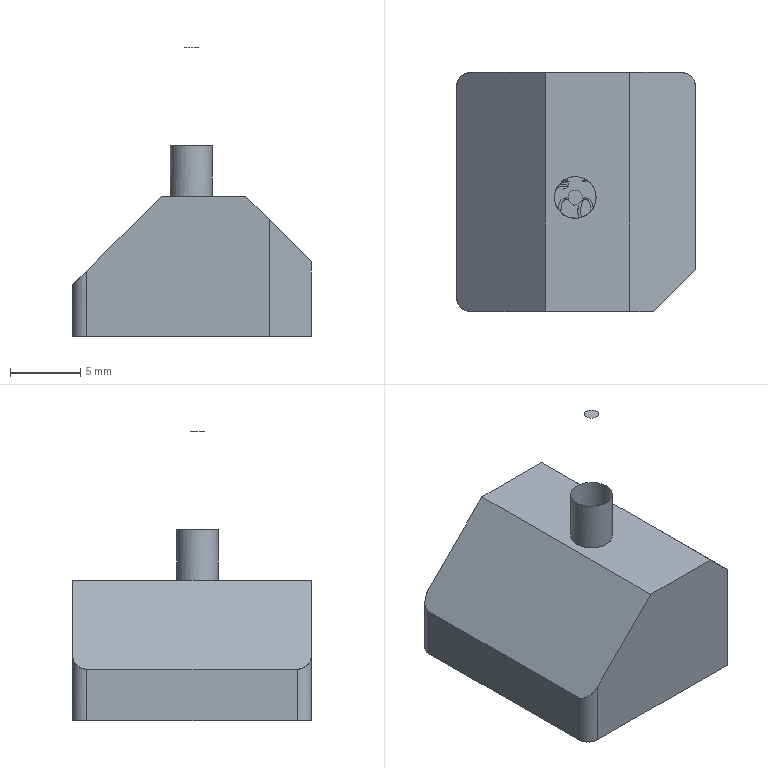NC program | PowerMill | posted with a generic post | part box 17 x 17 x 20.603 mm
Lines 1 to 1061 of 69435:
%
O0001
N104 ( POWERMILL CB  : 2026004.0)
N105 ( POST VER      : 2026.0.0.5161)
N106 ( OPTION FILE   : FANUC)
N107 ( OUTPUT WORKPLANE : WORLD)
N108 (  )
N109 ( TOOL LIST )
N110 (---------------------------------------)
N111 ( NO. | ID        | DIA.| TIP RAD|LENGTH)
N112 (---------------------------------------)
N113 (    1|D10C_1_1_1 |10.0 |  0.0   |76.04 )
N114 (    3|D10_1_1_1  |10.0 |  0.0   |75.76 )
N115 (   14|D4_1_1     | 4.0 |  0.0   |65.76 )
N116 (    7|R2_1_1     | 4.0 |  2.0   | 73.2 )
N117 (   13|TEXT_D4_1_1| 4.0 |  0.3   |65.88 )
N118 (---------------------------------------)
N119 (  )
N120 ( NUMBER OF TOOLPATHS: 10.0 )
N121 ( ESTIMATED PROGRAM DURATION: 0 HOURS 6 MIN 42 SEC)
N122 (  )
N123 G00 G21 G80 G40 G17
N124 G90
N125 G54
N126 G53 Z0.0
N127 (---------------)
N128 ( START TOOLPATH : 精公开粗01-扫面平行-D10C )
N129 (---------------)
N130 ( TOOL NO.    :1 )
N131 ( TOOL TYPE   : ENDMILL)
N132 ( TOOL ID     : D10C_1_1_1)
N133 ( TOOL DIA    : 10.0 LENGTH 76.04)
N134 T1
N135 M6
N136 S8000 M03
N137 G00 G90 X0.002 Y0.0
N138 G43 Z10.2 H1
N139
N140 G05 P10000 R4
N141 X16.302 Y11.3
N142 Z1.153
N143 G01 Z-0.047 F6000.0
N144 X11.302 F10000.0
N145 X-11.298
N146 Y5.65
N147 X11.302
N148 Y0.0
N149 X-11.298
N150 Y-5.65
N151 X11.302
N152 Y-11.3
N153 X-11.298
N154 X-16.298
N155 G00 Z10.2
N156 G05 P0
N157 (---------------)
N158 ( END TOOLPATH : 精公开粗01-扫面平行-D10C )
N159 (---------------)
N160 ( START TOOLPATH : 精公开粗01-外形偏置-D10C )
N161 (---------------)
N162 G00 X0.002 Y0.0 Z9.903
N163 G05 P10000 R4
N164 X5.2155 Y-16.575
N165 Z0.7136
N166 G01 Z-0.4864 F6000.0
N167 Y-16.0475 F10000.0
N168 G03 X0.468 Y-11.3 I-4.7475 J0.0
N169 G01 X-10.298
N170 G02 X-11.298 Y-10.3 I0.0 J1.0
N171 G01 Y10.3
N172 G02 X-10.298 Y11.3 I1.0 J0.0
N173 G01 X10.302
N174 G02 X11.302 Y10.3 I0.0 J-1.0
N175 G01 Y-10.3
N176 G02 X10.302 Y-11.3 I-1.0 J0.0
N177 G01 X0.468
N178 X0.3887 Y-6.22
N179 X-0.3847 Y-6.2321
N180 X-1.1581 Y-6.1315
N181 X-1.9316 Y-5.9309
N182 X-2.2756 Y-5.8007
N183 X-2.705 Y-5.5991
N184 X-3.4784 Y-5.1313
N185 X-4.2518 Y-4.4575
N186 X-4.4418 Y-4.2538
N187 X-5.0102 Y-3.4804
N188 X-5.4189 Y-2.707
N189 X-5.684 Y-1.9336
N190 X-5.8444 Y-1.1601
N191 X-5.889 Y-0.3867
N192 X-5.8408 Y0.3867
N193 X-5.6766 Y1.1601
N194 X-5.4075 Y1.9336
N195 X-5.0253 Y2.6552
N196 X-4.4176 Y3.4804
N197 X-4.2518 Y3.6568
N198 X-3.5825 Y4.2538
N199 X-2.705 Y4.7989
N200 X-1.9316 Y5.1308
N201 X-1.1581 Y5.3315
N202 X-0.3847 Y5.4321
N203 X0.3887 Y5.42
N204 X1.1621 Y5.3138
N205 X1.9356 Y5.0877
N206 X2.709 Y4.7473
N207 X3.4724 Y4.2538
N208 X4.2558 Y3.5415
N209 X4.894 Y2.707
N210 X5.2973 Y1.9336
N211 X5.5769 Y1.1601
N212 X5.7309 Y0.3867
N213 X5.7892 Y-0.3867
N214 X5.7346 Y-1.1601
N215 X5.5841 Y-1.9336
N216 X5.3099 Y-2.707
N217 X4.9107 Y-3.4804
N218 X4.3331 Y-4.2538
N219 X3.508 Y-5.0273
N220 X2.709 Y-5.5476
N221 X2.1672 Y-5.8007
N222 X1.1621 Y-6.1139
N223 X0.3887 Y-6.22
N224 X0.468 Y-11.3
N225 G00 Z3.3243
N226 G01 X5.2155 Y-16.575
N227 G00 Z0.3243
N228 G01 Z-0.8757 F6000.0
N229 Y-16.0475 F10000.0
N230 G03 X0.468 Y-11.3 I-4.7475 J0.0
N231 G01 X-10.298
N232 G02 X-11.298 Y-10.3 I0.0 J1.0
N233 G01 Y10.3
N234 G02 X-10.298 Y11.3 I1.0 J0.0
N235 G01 X10.302
N236 G02 X11.302 Y10.3 I0.0 J-1.0
N237 G01 Y-10.3
N238 G02 X10.302 Y-11.3 I-1.0 J0.0
N239 G01 X0.47
N240 X0.3887 Y-6.2744
N241 X-0.3847 Y-6.2869
N242 X-1.1581 Y-6.1868
N243 X-1.9316 Y-5.9885
N244 X-2.4138 Y-5.8007
N245 X-2.705 Y-5.6602
N246 X-3.4784 Y-5.1988
N247 X-3.7048 Y-5.0273
N248 X-4.2518 Y-4.5338
N249 X-4.514 Y-4.2538
N250 X-5.0253 Y-3.5593
N251 X-5.478 Y-2.707
N252 X-5.7402 Y-1.9336
N253 X-5.8995 Y-1.1601
N254 X-5.9432 Y-0.3867
N255 X-5.896 Y0.3867
N256 X-5.7987 Y0.9095
N257 X-5.4671 Y1.9336
N258 X-5.0573 Y2.707
N259 X-4.4901 Y3.4804
N260 X-4.2518 Y3.7337
N261 X-3.6709 Y4.2538
N262 X-3.4784 Y4.3979
N263 X-2.705 Y4.8597
N264 X-2.3533 Y5.0273
N265 X-1.9316 Y5.1882
N266 X-1.1581 Y5.3868
N267 X-0.3847 Y5.4869
N268 X0.3887 Y5.4744
N269 X1.1621 Y5.3695
N270 X1.9356 Y5.1452
N271 X2.2472 Y5.0273
N272 X2.709 Y4.809
N273 X3.4824 Y4.3143
N274 X4.2558 Y3.6223
N275 X4.9581 Y2.707
N276 X5.3562 Y1.9336
N277 X5.6333 Y1.1601
N278 X5.7856 Y0.3867
N279 X5.8439 Y-0.3867
N280 X5.8027 Y-1.0591
N281 X5.6405 Y-1.9336
N282 X5.3687 Y-2.707
N283 X5.0293 Y-3.3898
N284 X4.4041 Y-4.2538
N285 X4.2558 Y-4.4219
N286 X3.5976 Y-5.0273
N287 X2.709 Y-5.6096
N288 X2.3098 Y-5.8007
N289 X1.9356 Y-5.9451
N290 X1.1621 Y-6.1696
N291 X0.3887 Y-6.2744
N292 X0.47 Y-11.3
N293 X0.468
N294 G00 Z2.9349
N295 G01 X5.2155 Y-16.575
N296 G00 Z-0.0651
N297 G01 Z-1.2651 F6000.0
N298 Y-16.0475 F10000.0
N299 G03 X0.468 Y-11.3 I-4.7475 J0.0
N300 G01 X-10.298
N301 G02 X-11.298 Y-10.3 I0.0 J1.0
N302 G01 Y10.3
N303 G02 X-10.298 Y11.3 I1.0 J0.0
N304 G01 X10.302
N305 G02 X11.302 Y10.3 I0.0 J-1.0
N306 G01 Y-10.3
N307 G02 X10.302 Y-11.3 I-1.0 J0.0
N308 G01 X0.472
N309 X0.3887 Y-6.3287
N310 X-0.3847 Y-6.3417
N311 X-1.1581 Y-6.2421
N312 X-1.9316 Y-6.0461
N313 X-2.5431 Y-5.8007
N314 X-3.4784 Y-5.2654
N315 X-3.7912 Y-5.0273
N316 X-4.2518 Y-4.6101
N317 X-4.5858 Y-4.2538
N318 X-5.0253 Y-3.6611
N319 X-5.5372 Y-2.707
N320 X-5.7965 Y-1.9336
N321 X-5.9547 Y-1.1601
N322 X-5.9974 Y-0.3867
N323 X-5.9512 Y0.3867
N324 X-5.7987 Y1.1257
N325 X-5.5266 Y1.9336
N326 X-5.1207 Y2.707
N327 X-4.5626 Y3.4804
N328 X-4.2518 Y3.8107
N329 X-3.7589 Y4.2538
N330 X-3.4784 Y4.4648
N331 X-2.705 Y4.9204
N332 X-1.9316 Y5.2456
N333 X-1.1581 Y5.4421
N334 X-0.3847 Y5.5417
N335 X0.3887 Y5.5287
N336 X1.1621 Y5.4252
N337 X1.9356 Y5.2027
N338 X2.3859 Y5.0273
N339 X2.709 Y4.8706
N340 X3.653 Y4.2538
N341 X4.2558 Y3.703
N342 X4.4529 Y3.4804
N343 X5.0221 Y2.707
N344 X5.4151 Y1.9336
N345 X5.6898 Y1.1601
N346 X5.8027 Y0.6452
N347 X5.8986 Y-0.3867
N348 X5.844 Y-1.1601
N349 X5.6969 Y-1.9336
N350 X5.4274 Y-2.707
N351 X5.0383 Y-3.4804
N352 X4.4751 Y-4.2538
N353 X4.2558 Y-4.5022
N354 X3.6863 Y-5.0273
N355 X3.4824 Y-5.1815
N356 X2.709 Y-5.6716
N357 X2.4438 Y-5.8007
N358 X1.9356 Y-6.0026
N359 X1.1621 Y-6.2253
N360 X0.3887 Y-6.3287
N361 X0.472 Y-11.3
N362 X0.468
N363 G00 Z2.5455
N364 G01 X5.2155 Y-16.575
N365 G00 Z-0.4545
N366 G01 Z-1.6545 F6000.0
N367 Y-16.0475 F10000.0
N368 G03 X0.468 Y-11.3 I-4.7475 J0.0
N369 G01 X-10.298
N370 G02 X-11.298 Y-10.3 I0.0 J1.0
N371 G01 Y10.3
N372 G02 X-10.298 Y11.3 I1.0 J0.0
N373 G01 X10.302
N374 G02 X11.302 Y10.3 I0.0 J-1.0
N375 G01 Y-10.3
N376 G02 X10.302 Y-11.3 I-1.0 J0.0
N377 G01 X0.4739
N378 X0.3887 Y-6.3831
N379 X-0.3847 Y-6.3965
N380 X-1.1581 Y-6.2975
N381 X-1.9316 Y-6.1036
N382 X-2.6679 Y-5.8007
N383 X-3.4784 Y-5.3317
N384 X-3.8772 Y-5.0273
N385 X-4.2518 Y-4.6864
N386 X-4.6576 Y-4.2538
N387 X-5.0253 Y-3.7615
N388 X-5.2001 Y-3.4804
N389 X-5.5963 Y-2.707
N390 X-5.7987 Y-2.1257
N391 X-6.0098 Y-1.1601
N392 X-6.0516 Y-0.3867
N393 X-6.0064 Y0.3867
N394 X-5.8454 Y1.1601
N395 X-5.5862 Y1.9336
N396 X-5.1841 Y2.707
N397 X-5.0253 Y2.9607
N398 X-4.6351 Y3.4804
N399 X-4.2518 Y3.8858
N400 X-3.8449 Y4.2538
N401 X-3.4784 Y4.5317
N402 X-2.705 Y4.9812
N403 X-1.9316 Y5.303
N404 X-1.1581 Y5.4974
N405 X-0.3847 Y5.5964
N406 X0.3887 Y5.5831
N407 X1.1621 Y5.4809
N408 X1.9356 Y5.2602
N409 X2.709 Y4.9322
N410 X3.4824 Y4.4477
N411 X3.7399 Y4.2538
N412 X4.2558 Y3.7825
N413 X4.5244 Y3.4804
N414 X5.0293 Y2.8007
N415 X5.474 Y1.9336
N416 X5.7463 Y1.1601
N417 X5.8951 Y0.3867
N418 X5.9534 Y-0.3867
N419 X5.8987 Y-1.1601
N420 X5.7533 Y-1.9336
N421 X5.4861 Y-2.707
N422 X5.1022 Y-3.4804
N423 X4.5461 Y-4.2538
N424 X4.2558 Y-4.5825
N425 X3.7727 Y-5.0273
N426 X3.4824 Y-5.2478
N427 X2.5734 Y-5.8007
N428 X1.9356 Y-6.06
N429 X1.1621 Y-6.281
N430 X0.3887 Y-6.3831
N431 X0.4739 Y-11.3
N432 X0.468
N433 G00 Z2.1562
N434 G01 X5.2155 Y-16.575
N435 G00 Z-0.8438
N436 G01 Z-2.0438 F6000.0
N437 Y-16.0475 F10000.0
N438 G03 X0.468 Y-11.3 I-4.7475 J0.0
N439 G01 X-10.298
N440 G02 X-11.298 Y-10.3 I0.0 J1.0
N441 G01 Y10.3
N442 G02 X-10.298 Y11.3 I1.0 J0.0
N443 G01 X10.302
N444 G02 X11.302 Y10.3 I0.0 J-1.0
N445 G01 Y-10.3
N446 G02 X10.302 Y-11.3 I-1.0 J0.0
N447 G01 X0.4757
N448 X0.3887 Y-6.4374
N449 X-0.3847 Y-6.4512
N450 X-1.1581 Y-6.3528
N451 X-1.9316 Y-6.1612
N452 X-2.705 Y-5.8423
N453 X-3.4784 Y-5.398
N454 X-3.9603 Y-5.0273
N455 X-4.2518 Y-4.7606
N456 X-4.7294 Y-4.2538
N457 X-5.0253 Y-3.8589
N458 X-5.2635 Y-3.4804
N459 X-5.6554 Y-2.707
N460 X-5.9089 Y-1.9336
N461 X-6.0649 Y-1.1601
N462 X-6.1058 Y-0.3867
N463 X-6.0615 Y0.3867
N464 X-5.9017 Y1.1601
N465 X-5.6453 Y1.9336
N466 X-5.2475 Y2.707
N467 X-5.0253 Y3.0598
N468 X-4.7076 Y3.4804
N469 X-4.2518 Y3.9601
N470 X-3.9295 Y4.2538
N471 X-3.4784 Y4.5986
N472 X-2.7357 Y5.0273
N473 X-1.9316 Y5.3604
N474 X-1.1581 Y5.5528
N475 X-0.3847 Y5.6512
N476 X0.3887 Y5.6374
N477 X1.1621 Y5.5366
N478 X1.9356 Y5.3177
N479 X2.6436 Y5.0273
N480 X3.4824 Y4.5141
N481 X3.8269 Y4.2538
N482 X4.2558 Y3.8607
N483 X4.594 Y3.4804
N484 X5.0293 Y2.9011
N485 X5.1502 Y2.707
N486 X5.533 Y1.9336
N487 X5.8028 Y1.1601
N488 X5.9498 Y0.3867
N489 X6.0081 Y-0.3867
N490 X5.9534 Y-1.1601
N491 X5.8027 Y-1.964
N492 X5.5449 Y-2.707
N493 X5.166 Y-3.4804
N494 X5.0293 Y-3.7012
N495 X4.6157 Y-4.2538
N496 X4.2558 Y-4.6609
N497 X3.8591 Y-5.0273
N498 X3.4824 Y-5.3142
N499 X2.6971 Y-5.8007
N500 X1.9356 Y-6.1175
N501 X1.1621 Y-6.3367
N502 X0.3887 Y-6.4374
N503 X0.4757 Y-11.3
N504 X0.468
N505 G00 Z1.7668
N506 G01 X5.2155 Y-16.575
N507 G00 Z-1.2332
N508 G01 Z-2.4332 F6000.0
N509 Y-16.0475 F10000.0
N510 G03 X0.468 Y-11.3 I-4.7475 J0.0
N511 G01 X-10.298
N512 G02 X-11.298 Y-10.3 I0.0 J1.0
N513 G01 Y10.3
N514 G02 X-10.298 Y11.3 I1.0 J0.0
N515 G01 X10.302
N516 G02 X11.302 Y10.3 I0.0 J-1.0
N517 G01 Y-10.3
N518 G02 X10.302 Y-11.3 I-1.0 J0.0
N519 G01 X0.4775
N520 X0.3887 Y-6.4917
N521 X-0.3847 Y-6.506
N522 X-1.1581 Y-6.4082
N523 X-1.9316 Y-6.2188
N524 X-2.705 Y-5.9029
N525 X-3.4784 Y-5.4643
N526 X-4.0434 Y-5.0273
N527 X-4.7999 Y-4.2538
N528 X-5.0253 Y-3.9552
N529 X-5.3268 Y-3.4804
N530 X-5.7146 Y-2.707
N531 X-5.9651 Y-1.9336
N532 X-6.12 Y-1.1601
N533 X-6.16 Y-0.3867
N534 X-6.1166 Y0.3867
N535 X-5.958 Y1.1601
N536 X-5.7041 Y1.9336
N537 X-5.3109 Y2.707
N538 X-5.0253 Y3.1548
N539 X-4.778 Y3.4804
N540 X-4.2518 Y4.0343
N541 X-4.0132 Y4.2538
N542 X-3.4784 Y4.6649
N543 X-2.8536 Y5.0273
N544 X-1.9316 Y5.4177
N545 X-1.1581 Y5.6081
N546 X-0.3847 Y5.706
N547 X0.3887 Y5.6917
N548 X1.1621 Y5.5923
N549 X1.9356 Y5.3752
N550 X2.709 Y5.0555
N551 X3.4824 Y4.5804
N552 X3.9127 Y4.2538
N553 X4.2558 Y3.9389
N554 X4.6637 Y3.4804
N555 X5.0293 Y2.9993
N556 X5.2143 Y2.707
N557 X5.5919 Y1.9336
N558 X5.8027 Y1.3637
N559 X6.0045 Y0.3867
N560 X6.0628 Y-0.3867
N561 X6.0081 Y-1.1601
N562 X5.8661 Y-1.9336
N563 X5.6036 Y-2.707
N564 X5.2298 Y-3.4804
N565 X5.0293 Y-3.7996
N566 X4.6853 Y-4.2538
N567 X4.2558 Y-4.7383
N568 X3.944 Y-5.0273
N569 X3.4824 Y-5.3806
N570 X2.8152 Y-5.8007
N571 X1.9356 Y-6.1749
N572 X1.1621 Y-6.3924
N573 X0.3887 Y-6.4917
N574 X0.4775 Y-11.3
N575 X0.468
N576 G00 Z1.3774
N577 G01 X5.2155 Y-16.575
N578 G00 Z-1.6226
N579 G01 Z-2.8226 F6000.0
N580 Y-16.0475 F10000.0
N581 G03 X0.468 Y-11.3 I-4.7475 J0.0
N582 G01 X-10.298
N583 G02 X-11.298 Y-10.3 I0.0 J1.0
N584 G01 Y10.3
N585 G02 X-10.298 Y11.3 I1.0 J0.0
N586 G01 X10.302
N587 G02 X11.302 Y10.3 I0.0 J-1.0
N588 G01 Y-10.3
N589 G02 X10.302 Y-11.3 I-1.0 J0.0
N590 G01 X0.4792
N591 X0.3887 Y-6.5461
N592 X-0.3847 Y-6.5608
N593 X-1.1581 Y-6.4635
N594 X-1.9316 Y-6.2762
N595 X-2.705 Y-5.9635
N596 X-3.4784 Y-5.5306
N597 X-4.1238 Y-5.0273
N598 X-4.8697 Y-4.2538
N599 X-5.3901 Y-3.4804
N600 X-5.7737 Y-2.707
N601 X-6.0213 Y-1.9336
N602 X-6.1751 Y-1.1601
N603 X-6.2142 Y-0.3867
N604 X-6.1717 Y0.3867
N605 X-6.0142 Y1.1601
N606 X-5.7987 Y1.8439
N607 X-5.3743 Y2.707
N608 X-5.0253 Y3.2498
N609 X-4.8482 Y3.4804
N610 X-4.2518 Y4.1086
N611 X-3.4784 Y4.7301
N612 X-2.705 Y5.1634
N613 X-1.9316 Y5.4751
N614 X-1.1581 Y5.6634
N615 X-0.3847 Y5.7608
N616 X0.3887 Y5.7461
N617 X1.1621 Y5.648
N618 X1.9356 Y5.4327
N619 X2.709 Y5.1171
N620 X3.4824 Y4.6467
N621 X3.9965 Y4.2538
N622 X4.2558 Y4.0158
N623 X4.7333 Y3.4804
N624 X5.0293 Y3.0948
N625 X5.2776 Y2.707
N626 X5.6508 Y1.9336
N627 X5.8027 Y1.5409
N628 X5.9157 Y1.1601
N629 X6.0593 Y0.3867
N630 X6.1175 Y-0.3867
N631 X6.0628 Y-1.1601
N632 X5.9225 Y-1.9336
N633 X5.8027 Y-2.3416
N634 X5.6624 Y-2.707
N635 X5.2929 Y-3.4804
N636 X5.0293 Y-3.8964
N637 X4.7549 Y-4.2538
N638 X4.2558 Y-4.8158
N639 X4.0271 Y-5.0273
N640 X3.4824 Y-5.4469
N641 X2.9292 Y-5.8007
N642 X2.709 Y-5.9163
N643 X1.9356 Y-6.2324
N644 X1.1621 Y-6.4481
N645 X0.3887 Y-6.5461
N646 X0.4792 Y-11.3
N647 X0.468
N648 G00 Z0.988
N649 G01 X5.2155 Y-16.575
N650 G00 Z-2.012
N651 G01 Z-3.212 F6000.0
N652 Y-16.0475 F10000.0
N653 G03 X0.468 Y-11.3 I-4.7475 J0.0
N654 G01 X0.3409
N655 X0.1627 Y-6.5949
N656 X-0.3847 Y-6.6156
N657 X-1.1581 Y-6.5189
N658 X-1.9316 Y-6.3331
N659 X-2.705 Y-6.0241
N660 X-3.4784 Y-5.596
N661 X-4.2036 Y-5.0273
N662 X-4.9394 Y-4.2538
N663 X-5.4535 Y-3.4804
N664 X-5.7987 Y-2.7919
N665 X-6.0775 Y-1.9336
N666 X-6.2301 Y-1.1601
N667 X-6.2684 Y-0.3867
N668 X-6.2269 Y0.3867
N669 X-6.0705 Y1.1601
N670 X-5.8216 Y1.9336
N671 X-5.4377 Y2.707
N672 X-4.9184 Y3.4804
N673 X-4.2518 Y4.1828
N674 X-3.4784 Y4.7953
N675 X-2.705 Y5.2242
N676 X-1.9316 Y5.5325
N677 X-1.1581 Y5.7188
N678 X-0.5961 Y5.8007
N679 X0.3824
N680 X1.1621 Y5.7037
N681 X1.9356 Y5.4902
N682 X2.709 Y5.1782
N683 X2.9935 Y5.0273
N684 X3.4824 Y4.7131
N685 X4.0802 Y4.2538
N686 X4.2558 Y4.0916
N687 X4.803 Y3.4804
N688 X5.0293 Y3.1904
N689 X5.3403 Y2.707
N690 X5.7097 Y1.9336
N691 X5.9722 Y1.1601
N692 X6.114 Y0.3867
N693 X6.1722 Y-0.3867
N694 X6.1175 Y-1.1601
N695 X5.9789 Y-1.9336
N696 X5.8027 Y-2.5046
N697 X5.3553 Y-3.4804
N698 X5.0293 Y-3.9895
N699 X4.8246 Y-4.2538
N700 X4.2558 Y-4.8923
N701 X3.4824 Y-5.5133
N702 X3.0404 Y-5.8007
N703 X2.709 Y-5.9774
N704 X1.9356 Y-6.2898
N705 X1.1621 Y-6.5038
N706 X0.7101 Y-6.5741
N707 X0.1627 Y-6.5949
N708 X0.3409 Y-11.3
N709 X-10.298
N710 G02 X-11.298 Y-10.3 I0.0 J1.0
N711 G01 Y10.3
N712 G02 X-10.298 Y11.3 I1.0 J0.0
N713 G01 X10.302
N714 G02 X11.302 Y10.3 I0.0 J-1.0
N715 G01 Y-10.3
N716 G02 X10.302 Y-11.3 I-1.0 J0.0
N717 G01 X0.468
N718 G00 Z0.5987
N719 G01 X5.2155 Y-16.575
N720 G00 Z-2.4013
N721 G01 Z-3.6013 F6000.0
N722 Y-16.0475 F10000.0
N723 G03 X0.468 Y-11.3 I-4.7475 J0.0
N724 G01 X-10.298
N725 G02 X-11.298 Y-10.3 I0.0 J1.0
N726 G01 Y10.3
N727 G02 X-10.298 Y11.3 I1.0 J0.0
N728 G01 X10.302
N729 G02 X11.302 Y10.3 I0.0 J-1.0
N730 G01 Y-10.3
N731 G02 X10.302 Y-11.3 I-1.0 J0.0
N732 G01 X0.4825
N733 X0.3887 Y-6.6548
N734 X-0.3847 Y-6.6704
N735 X-1.159 Y-6.5741
N736 X-1.9316 Y-6.39
N737 X-2.705 Y-6.0848
N738 X-3.4784 Y-5.6606
N739 X-4.2518 Y-5.0576
N740 X-5.0092 Y-4.2538
N741 X-5.5168 Y-3.4804
N742 X-5.892 Y-2.707
N743 X-6.1337 Y-1.9336
N744 X-6.2852 Y-1.1601
N745 X-6.3226 Y-0.3867
N746 X-6.282 Y0.3867
N747 X-6.1268 Y1.1601
N748 X-5.8804 Y1.9336
N749 X-5.5011 Y2.707
N750 X-5.0253 Y3.4329
N751 X-4.2557 Y4.2538
N752 X-3.4784 Y4.8604
N753 X-2.705 Y5.2849
N754 X-1.9316 Y5.5899
N755 X-1.1581 Y5.7741
N756 X-0.3847 Y5.8703
N757 X0.3887 Y5.8548
N758 X1.1621 Y5.7594
N759 X1.9356 Y5.5477
N760 X2.709 Y5.2386
N761 X3.1025 Y5.0273
N762 X3.4824 Y4.7794
N763 X4.2558 Y4.1674
N764 X5.0293 Y3.2812
N765 X5.4029 Y2.707
N766 X5.7686 Y1.9336
N767 X6.0287 Y1.1601
N768 X6.1687 Y0.3867
N769 X6.2269 Y-0.3867
N770 X6.1722 Y-1.1601
N771 X6.0353 Y-1.9336
N772 X5.8027 Y-2.6544
N773 X5.4177 Y-3.4804
N774 X5.0293 Y-4.0823
N775 X4.2558 Y-4.9673
N776 X3.4824 Y-5.5797
N777 X3.1468 Y-5.8007
N778 X2.709 Y-6.0386
N779 X1.9356 Y-6.3472
N780 X1.0906 Y-6.5741
N781 X0.3887 Y-6.6548
N782 X0.4825 Y-11.3
N783 X0.468
N784 G00 Z0.2093
N785 G01 X5.2155 Y-16.575
N786 G00 Z-2.7907
N787 G01 Z-3.9907 F6000.0
N788 Y-16.0475 F10000.0
N789 G03 X0.468 Y-11.3 I-4.7475 J0.0
N790 G01 X-10.298
N791 G02 X-11.298 Y-10.3 I0.0 J1.0
N792 G01 Y10.3
N793 G02 X-10.298 Y11.3 I1.0 J0.0
N794 G01 X10.302
N795 G02 X11.302 Y10.3 I0.0 J-1.0
N796 G01 Y-10.3
N797 G02 X10.302 Y-11.3 I-1.0 J0.0
N798 G01 X0.484
N799 X0.3887 Y-6.7091
N800 X-0.3847 Y-6.7252
N801 X-1.1581 Y-6.6295
N802 X-1.9316 Y-6.4468
N803 X-2.705 Y-6.1454
N804 X-3.3563 Y-5.8007
N805 X-4.2518 Y-5.1311
N806 X-5.0253 Y-4.3222
N807 X-5.5801 Y-3.4804
N808 X-5.7987 Y-3.0626
N809 X-5.9501 Y-2.707
N810 X-6.1899 Y-1.9336
N811 X-6.3403 Y-1.1601
N812 X-6.3768 Y-0.3867
N813 X-6.3371 Y0.3867
N814 X-6.183 Y1.1601
N815 X-5.9392 Y1.9336
N816 X-5.7987 Y2.2623
N817 X-5.5645 Y2.707
N818 X-5.0579 Y3.4804
N819 X-4.3351 Y4.2538
N820 X-3.4784 Y4.9256
N821 X-2.705 Y5.3457
N822 X-1.9316 Y5.6473
N823 X-1.2976 Y5.8007
N824 X-0.3847 Y5.9251
N825 X0.3887 Y5.9091
N826 X1.1621 Y5.8151
N827 X1.9356 Y5.6052
N828 X2.709 Y5.299
N829 X3.2084 Y5.0273
N830 X3.4824 Y4.8458
N831 X4.2433 Y4.2538
N832 X4.9423 Y3.4804
N833 X5.4655 Y2.707
N834 X5.8027 Y1.9948
N835 X6.0852 Y1.1601
N836 X6.2234 Y0.3867
N837 X6.2816 Y-0.3867
N838 X6.2269 Y-1.1601
N839 X6.0917 Y-1.9336
N840 X5.8386 Y-2.707
N841 X5.4801 Y-3.4804
N842 X5.0293 Y-4.1713
N843 X4.2721 Y-5.0273
N844 X3.4824 Y-5.6461
N845 X3.2505 Y-5.8007
N846 X2.709 Y-6.0998
N847 X1.9356 Y-6.4047
N848 X1.3603 Y-6.5741
N849 X0.3887 Y-6.7091
N850 X0.484 Y-11.3
N851 X0.468
N852 G00 Z-0.1801
N853 G01 X5.2155 Y-16.575
N854 G00 Z-3.1801
N855 G01 Z-4.3801 F6000.0
N856 Y-16.0475 F10000.0
N857 G03 X0.468 Y-11.3 I-4.7475 J0.0
N858 G01 X-10.298
N859 G02 X-11.298 Y-10.3 I0.0 J1.0
N860 G01 Y10.3
N861 G02 X-10.298 Y11.3 I1.0 J0.0
N862 G01 X10.302
N863 G02 X11.302 Y10.3 I0.0 J-1.0
N864 G01 Y-10.3
N865 G02 X10.302 Y-11.3 I-1.0 J0.0
N866 G01 X0.4855
N867 X0.3887 Y-6.7634
N868 X-0.3847 Y-6.7799
N869 X-1.1581 Y-6.6849
N870 X-1.9316 Y-6.5037
N871 X-2.705 Y-6.206
N872 X-3.4615 Y-5.8007
N873 X-4.2518 Y-5.2043
N874 X-5.0253 Y-4.4108
N875 X-5.6425 Y-3.4804
N876 X-5.7987 Y-3.1897
N877 X-6.0082 Y-2.707
N878 X-6.2461 Y-1.9336
N879 X-6.3954 Y-1.1601
N880 X-6.4309 Y-0.3867
N881 X-6.3922 Y0.3867
N882 X-6.2393 Y1.1601
N883 X-5.998 Y1.9336
N884 X-5.7987 Y2.3892
N885 X-5.6272 Y2.707
N886 X-5.0253 Y3.6102
N887 X-4.2518 Y4.4053
N888 X-3.4784 Y4.9907
N889 X-2.705 Y5.4064
N890 X-1.9316 Y5.7046
N891 X-1.1581 Y5.8847
N892 X-0.3847 Y5.9799
N893 X0.3887 Y5.9634
N894 X1.1621 Y5.8707
N895 X1.4811 Y5.8007
N896 X1.9356 Y5.6627
N897 X2.709 Y5.3594
N898 X3.3101 Y5.0273
N899 X4.2558 Y4.3168
N900 X5.0293 Y3.4605
N901 X5.5281 Y2.707
N902 X5.8027 Y2.1309
N903 X6.1417 Y1.1601
N904 X6.2781 Y0.3867
N905 X6.3364 Y-0.3867
N906 X6.2816 Y-1.1601
N907 X6.1481 Y-1.9336
N908 X5.8973 Y-2.707
N909 X5.5425 Y-3.4804
N910 X5.0293 Y-4.2602
N911 X4.3524 Y-5.0273
N912 X3.4824 Y-5.7124
N913 X2.709 Y-6.1602
N914 X1.9356 Y-6.4621
N915 X1.5817 Y-6.5741
N916 X1.1621 Y-6.671
N917 X0.3887 Y-6.7634
N918 X0.4855 Y-11.3
N919 X0.468
N920 G00 Z-0.5694
N921 G01 X5.2155 Y-16.575
N922 G00 Z-3.5694
N923 G01 Z-4.7694 F6000.0
N924 Y-16.0475 F10000.0
N925 G03 X0.468 Y-11.3 I-4.7475 J0.0
N926 G01 X-10.298
N927 G02 X-11.298 Y-10.3 I0.0 J1.0
N928 G01 Y10.3
N929 G02 X-10.298 Y11.3 I1.0 J0.0
N930 G01 X10.302
N931 G02 X11.302 Y10.3 I0.0 J-1.0
N932 G01 Y-10.3
N933 G02 X10.302 Y-11.3 I-1.0 J0.0
N934 G01 X0.4869
N935 X0.3887 Y-6.8178
N936 X-0.3847 Y-6.8347
N937 X-1.1581 Y-6.7402
N938 X-1.8885 Y-6.5741
N939 X-2.705 Y-6.2666
N940 X-3.4784 Y-5.8543
N941 X-4.2518 Y-5.2775
N942 X-4.5224 Y-5.0273
N943 X-5.0253 Y-4.4967
N944 X-5.214 Y-4.2538
N945 X-5.7047 Y-3.4804
N946 X-6.0662 Y-2.707
N947 X-6.3024 Y-1.9336
N948 X-6.4505 Y-1.1601
N949 X-6.4851 Y-0.3867
N950 X-6.4473 Y0.3867
N951 X-6.2956 Y1.1601
N952 X-6.0568 Y1.9336
N953 X-5.7987 Y2.5092
N954 X-5.1943 Y3.4804
N955 X-5.0253 Y3.6973
N956 X-4.2518 Y4.4779
N957 X-3.5226 Y5.0273
N958 X-2.705 Y5.4669
N959 X-1.9316 Y5.7619
N960 X-1.1581 Y5.9401
N961 X-0.3847 Y6.0346
N962 X0.3887 Y6.0178
N963 X1.1621 Y5.9264
N964 X1.6877 Y5.8007
N965 X2.709 Y5.4198
N966 X3.4101 Y5.0273
N967 X4.2558 Y4.3901
N968 X4.4036 Y4.2538
N969 X5.0293 Y3.5469
N970 X5.5907 Y2.707
N971 X5.9454 Y1.9336
N972 X6.1981 Y1.1601
N973 X6.3329 Y0.3867
N974 X6.3911 Y-0.3867
N975 X6.3363 Y-1.1601
N976 X6.2045 Y-1.9336
N977 X5.9561 Y-2.707
N978 X5.6048 Y-3.4804
N979 X5.1031 Y-4.2538
N980 X4.4307 Y-5.0273
N981 X4.2558 Y-5.1905
N982 X3.4494 Y-5.8007
N983 X2.709 Y-6.2201
N984 X1.7739 Y-6.5741
N985 X1.1621 Y-6.7267
N986 X0.3887 Y-6.8178
N987 X0.4869 Y-11.3
N988 X0.468
N989 G00 Z-0.9588
N990 G01 X5.2155 Y-16.575
N991 G00 Z-3.9588
N992 G01 Z-5.1588 F6000.0
N993 Y-16.0475 F10000.0
N994 G03 X0.468 Y-11.3 I-4.7475 J0.0
N995 G01 X-10.298
N996 G02 X-11.298 Y-10.3 I0.0 J1.0
N997 G01 Y10.3
N998 G02 X-10.298 Y11.3 I1.0 J0.0
N999 G01 X10.302
N1000 G02 X11.302 Y10.3 I0.0 J-1.0
N1001 G01 Y-10.3
N1002 G02 X10.302 Y-11.3 I-1.0 J0.0
N1003 G01 X0.4882
N1004 X0.3887 Y-6.8721
N1005 X-0.3847 Y-6.8895
N1006 X-1.1581 Y-6.7956
N1007 X-1.9316 Y-6.6175
N1008 X-2.705 Y-6.3272
N1009 X-3.6644 Y-5.8007
N1010 X-4.2518 Y-5.3507
N1011 X-4.6016 Y-5.0273
N1012 X-5.0253 Y-4.5826
N1013 X-5.2818 Y-4.2538
N1014 X-5.767 Y-3.4804
N1015 X-6.1243 Y-2.707
N1016 X-6.3586 Y-1.9336
N1017 X-6.5055 Y-1.1601
N1018 X-6.5393 Y-0.3867
N1019 X-6.5025 Y0.3867
N1020 X-6.3519 Y1.1601
N1021 X-6.1156 Y1.9336
N1022 X-5.7987 Y2.625
N1023 X-5.2626 Y3.4804
N1024 X-5.0253 Y3.782
N1025 X-4.5734 Y4.2538
N1026 X-4.2518 Y4.5504
N1027 X-3.6238 Y5.0273
N1028 X-2.705 Y5.5267
N1029 X-1.9914 Y5.8007
N1030 X-1.1581 Y5.9954
N1031 X-0.3847 Y6.0894
N1032 X0.3887 Y6.0721
N1033 X1.1621 Y5.9821
N1034 X1.8678 Y5.8007
N1035 X2.709 Y5.4802
N1036 X3.4824 Y5.0439
N1037 X4.2558 Y4.4634
N1038 X4.4815 Y4.2538
N1039 X5.1513 Y3.4804
N1040 X5.6529 Y2.707
N1041 X6.0043 Y1.9336
N1042 X6.2546 Y1.1601
N1043 X6.3876 Y0.3867
N1044 X6.4458 Y-0.3867
N1045 X6.3911 Y-1.1601
N1046 X6.2609 Y-1.9336
N1047 X6.0148 Y-2.707
N1048 X5.667 Y-3.4804
N1049 X5.1724 Y-4.2538
N1050 X4.5084 Y-5.0273
N1051 X4.2558 Y-5.2633
N1052 X3.5453 Y-5.8007
N1053 X2.709 Y-6.2799
N1054 X1.9465 Y-6.5741
N1055 X1.1621 Y-6.7824
N1056 X0.3887 Y-6.8721
N1057 X0.4882 Y-11.3
N1058 X0.468
N1059 G00 Z-1.3482
N1060 G01 X5.2155 Y-16.575
N1061 G00 Z-4.3482
N1062 G01 Z-5.5482 F6000.0
N1063 Y-16.0475 F10000.0
N1064 G03 X0.468 Y-11.3 I-4.7475 J0.0
N1065 G01 X-10.298
N1066 G02 X-11.298 Y-10.3 I0.0 J1.0
N1067 G01 Y10.3
N1068 G02 X-10.298 Y11.3 I1.0 J0.0
N1069 G01 X10.302
N1070 G02 X11.302 Y10.3 I0.0 J-1.0
N1071 G01 Y-10.3
N1072 G02 X10.302 Y-11.3 I-1.0 J0.0
N1073 G01 X0.4895
N1074 X0.3887 Y-6.9265
N1075 X-0.3847 Y-6.9443
N1076 X-1.1581 Y-6.8509
N1077 X-1.9316 Y-6.6744
N1078 X-2.2472 Y-6.5741
N1079 X-2.705 Y-6.387
N1080 X-3.4784 Y-5.9815
N1081 X-3.7635 Y-5.8007
N1082 X-4.2518 Y-5.4239
N1083 X-4.68 Y-5.0273
N1084 X-5.0253 Y-4.6659
N1085 X-5.3496 Y-4.2538
N1086 X-5.7987 Y-3.5363
N1087 X-6.1824 Y-2.707
N1088 X-6.4148 Y-1.9336
N1089 X-6.5606 Y-1.1601
N1090 X-6.5935 Y-0.3867
N1091 X-6.5721 Y0.2466
N1092 X-6.4081 Y1.1601
N1093 X-6.174 Y1.9336
N1094 X-5.8144 Y2.707
N1095 X-5.3306 Y3.4804
N1096 X-5.0253 Y3.8667
N1097 X-4.6528 Y4.2538
N1098 X-4.2518 Y4.623
N1099 X-3.7239 Y5.0273
N1100 X-3.4784 Y5.1813
N1101 X-2.705 Y5.5866
N1102 X-1.9316 Y5.8754
N1103 X-1.1581 Y6.0507
N1104 X-0.3847 Y6.1442
N1105 X0.3887 Y6.1265
N1106 X1.1621 Y6.0378
N1107 X1.9356 Y5.8353
N1108 X2.709 Y5.5406
N1109 X3.4824 Y5.109
N1110 X4.2558 Y4.5364
N1111 X4.5594 Y4.2538
N1112 X5.2206 Y3.4804
N1113 X5.714 Y2.707
N1114 X6.0632 Y1.9336
N1115 X6.3111 Y1.1601
N1116 X6.4423 Y0.3867
N1117 X6.5005 Y-0.3867
N1118 X6.4458 Y-1.1601
N1119 X6.3173 Y-1.9336
N1120 X6.0735 Y-2.707
N1121 X5.8027 Y-3.3305
N1122 X5.2401 Y-4.2538
N1123 X4.586 Y-5.0273
N1124 X4.2558 Y-5.3361
N1125 X3.4824 Y-5.9098
N1126 X2.709 Y-6.3398
N1127 X2.1084 Y-6.5741
N1128 X1.1621 Y-6.8381
N1129 X0.3887 Y-6.9265
N1130 X0.4895 Y-11.3
N1131 X0.468
N1132 G00 Z-1.7376
N1133 G01 X5.2155 Y-16.575
N1134 G00 Z-4.7376
N1135 G01 Z-5.9376 F6000.0
N1136 Y-16.0475 F10000.0
N1137 G03 X0.468 Y-11.3 I-4.7475 J0.0
N1138 G01 X-10.298
N1139 G02 X-11.298 Y-10.3 I0.0 J1.0
N1140 G01 Y10.3
N1141 G02 X-10.298 Y11.3 I1.0 J0.0
N1142 G01 X10.302
N1143 G02 X11.302 Y10.3 I0.0 J-1.0
N1144 G01 Y-10.3
N1145 G02 X10.302 Y-11.3 I-1.0 J0.0
N1146 G01 X0.4907
N1147 X0.3887 Y-6.9808
N1148 X-0.3847 Y-6.9991
N1149 X-1.1581 Y-6.9062
N1150 X-1.9316 Y-6.7312
N1151 X-2.4044 Y-6.5741
N1152 X-2.705 Y-6.4468
N1153 X-3.4784 Y-6.0443
N1154 X-3.8586 Y-5.8007
N1155 X-4.2518 Y-5.4949
N1156 X-4.7583 Y-5.0273
N1157 X-5.0253 Y-4.7488
N1158 X-5.4154 Y-4.2538